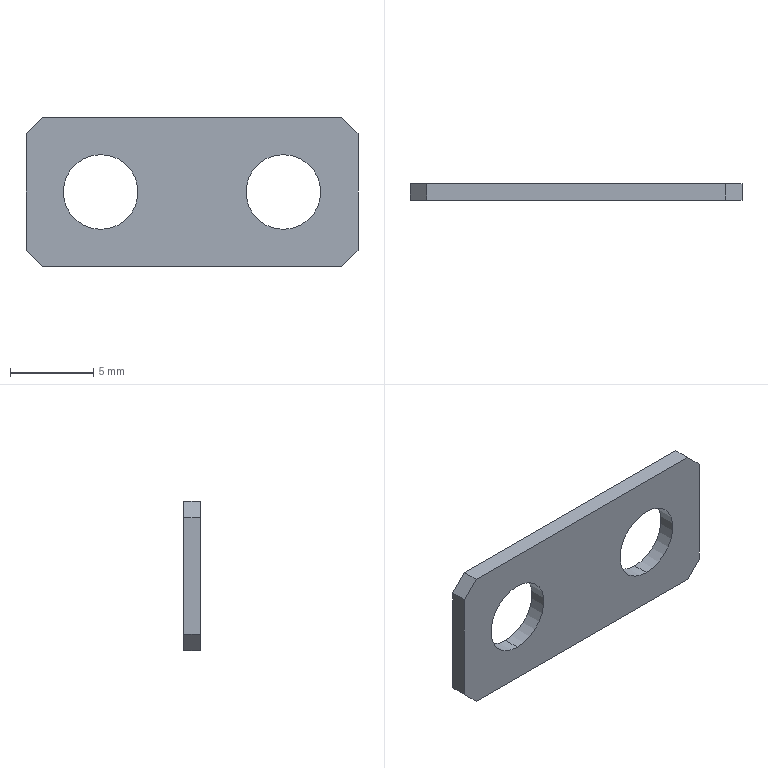Part | STEP file | 10000054028swp000-1 | 1 solid | 14 faces | box 20 x 1 x 9 mm | volume 146.191 mm3 | plane 10 | cylinder 4 | commonest cylinder face diameters 4.5 x4
STEP:
#1=CARTESIAN_POINT('',(-5.5,-0.5,-2.25));
#2=VERTEX_POINT('',#1);
#3=CARTESIAN_POINT('',(-5.5,-0.5,2.25));
#4=VERTEX_POINT('',#3);
#5=CARTESIAN_POINT('',(-5.5,-0.5,0.));
#6=DIRECTION('',(0.,1.,0.));
#7=DIRECTION('',(0.,0.,1.));
#8=AXIS2_PLACEMENT_3D('',#5,#6,#7);
#9=CIRCLE('',#8,2.25);
#10=EDGE_CURVE('',#2,#4,#9,.T.);
#11=ORIENTED_EDGE('',*,*,#10,.F.);
#12=CARTESIAN_POINT('',(-5.5,0.5,-2.25));
#13=VERTEX_POINT('',#12);
#14=CARTESIAN_POINT('',(-5.5,0.5,-2.25));
#15=DIRECTION('',(0.,1.,0.));
#16=VECTOR('',#15,1000.);
#17=LINE('',#14,#16);
#18=EDGE_CURVE('',#2,#13,#17,.T.);
#19=ORIENTED_EDGE('',*,*,#18,.T.);
#20=CARTESIAN_POINT('',(-5.5,0.5,2.25));
#21=VERTEX_POINT('',#20);
#22=CARTESIAN_POINT('',(-5.5,0.5,0.));
#23=DIRECTION('',(0.,1.,0.));
#24=DIRECTION('',(0.,0.,1.));
#25=AXIS2_PLACEMENT_3D('',#22,#23,#24);
#26=CIRCLE('',#25,2.25);
#27=EDGE_CURVE('',#13,#21,#26,.T.);
#28=ORIENTED_EDGE('',*,*,#27,.T.);
#29=CARTESIAN_POINT('',(-5.5,0.5,2.25));
#30=DIRECTION('',(0.,1.,0.));
#31=VECTOR('',#30,1000.);
#32=LINE('',#29,#31);
#33=EDGE_CURVE('',#4,#21,#32,.T.);
#34=ORIENTED_EDGE('',*,*,#33,.F.);
#35=EDGE_LOOP('',(#11,#19,#28,#34));
#36=FACE_OUTER_BOUND('',#35,.T.);
#37=CARTESIAN_POINT('',(-5.5,0.5,0.));
#38=DIRECTION('',(0.,1.,0.));
#39=DIRECTION('',(0.,0.,1.));
#40=AXIS2_PLACEMENT_3D('',#37,#38,#39);
#41=CYLINDRICAL_SURFACE('',#40,2.25);
#42=ADVANCED_FACE('',(#36),#41,.F.);
#43=CARTESIAN_POINT('',(5.5,-0.5,-2.25));
#44=VERTEX_POINT('',#43);
#45=CARTESIAN_POINT('',(5.5,-0.5,2.25));
#46=VERTEX_POINT('',#45);
#47=CARTESIAN_POINT('',(5.5,-0.5,0.));
#48=DIRECTION('',(0.,1.,0.));
#49=DIRECTION('',(0.,0.,1.));
#50=AXIS2_PLACEMENT_3D('',#47,#48,#49);
#51=CIRCLE('',#50,2.25);
#52=EDGE_CURVE('',#44,#46,#51,.T.);
#53=ORIENTED_EDGE('',*,*,#52,.F.);
#54=CARTESIAN_POINT('',(5.5,0.5,-2.25));
#55=VERTEX_POINT('',#54);
#56=CARTESIAN_POINT('',(5.5,0.5,-2.25));
#57=DIRECTION('',(0.,1.,0.));
#58=VECTOR('',#57,1000.);
#59=LINE('',#56,#58);
#60=EDGE_CURVE('',#44,#55,#59,.T.);
#61=ORIENTED_EDGE('',*,*,#60,.T.);
#62=CARTESIAN_POINT('',(5.5,0.5,2.25));
#63=VERTEX_POINT('',#62);
#64=CARTESIAN_POINT('',(5.5,0.5,0.));
#65=DIRECTION('',(0.,1.,0.));
#66=DIRECTION('',(0.,0.,1.));
#67=AXIS2_PLACEMENT_3D('',#64,#65,#66);
#68=CIRCLE('',#67,2.25);
#69=EDGE_CURVE('',#55,#63,#68,.T.);
#70=ORIENTED_EDGE('',*,*,#69,.T.);
#71=CARTESIAN_POINT('',(5.5,0.5,2.25));
#72=DIRECTION('',(0.,1.,0.));
#73=VECTOR('',#72,1000.);
#74=LINE('',#71,#73);
#75=EDGE_CURVE('',#46,#63,#74,.T.);
#76=ORIENTED_EDGE('',*,*,#75,.F.);
#77=EDGE_LOOP('',(#53,#61,#70,#76));
#78=FACE_OUTER_BOUND('',#77,.T.);
#79=CARTESIAN_POINT('',(5.5,0.5,0.));
#80=DIRECTION('',(0.,1.,0.));
#81=DIRECTION('',(0.,0.,1.));
#82=AXIS2_PLACEMENT_3D('',#79,#80,#81);
#83=CYLINDRICAL_SURFACE('',#82,2.25);
#84=ADVANCED_FACE('',(#78),#83,.F.);
#85=CARTESIAN_POINT('',(10.,-0.5,3.5));
#86=VERTEX_POINT('',#85);
#87=CARTESIAN_POINT('',(10.,-0.5,-3.5));
#88=VERTEX_POINT('',#87);
#89=CARTESIAN_POINT('',(10.,-0.5,-4.5));
#90=DIRECTION('',(0.,0.,-1.));
#91=VECTOR('',#90,1000.);
#92=LINE('',#89,#91);
#93=EDGE_CURVE('',#86,#88,#92,.T.);
#94=ORIENTED_EDGE('',*,*,#93,.T.);
#95=CARTESIAN_POINT('',(10.,0.5,-3.5));
#96=VERTEX_POINT('',#95);
#97=CARTESIAN_POINT('',(10.,0.5,-3.5));
#98=DIRECTION('',(0.,1.,0.));
#99=VECTOR('',#98,1000.);
#100=LINE('',#97,#99);
#101=EDGE_CURVE('',#88,#96,#100,.T.);
#102=ORIENTED_EDGE('',*,*,#101,.T.);
#103=CARTESIAN_POINT('',(10.,0.5,3.5));
#104=VERTEX_POINT('',#103);
#105=CARTESIAN_POINT('',(10.,0.5,-4.5));
#106=DIRECTION('',(0.,0.,-1.));
#107=VECTOR('',#106,1000.);
#108=LINE('',#105,#107);
#109=EDGE_CURVE('',#104,#96,#108,.T.);
#110=ORIENTED_EDGE('',*,*,#109,.F.);
#111=CARTESIAN_POINT('',(10.,0.5,3.5));
#112=DIRECTION('',(0.,-1.,0.));
#113=VECTOR('',#112,1000.);
#114=LINE('',#111,#113);
#115=EDGE_CURVE('',#104,#86,#114,.T.);
#116=ORIENTED_EDGE('',*,*,#115,.T.);
#117=EDGE_LOOP('',(#94,#102,#110,#116));
#118=FACE_OUTER_BOUND('',#117,.T.);
#119=CARTESIAN_POINT('',(10.,0.5,-4.5));
#120=DIRECTION('',(-1.,0.,0.));
#121=DIRECTION('',(0.,0.,1.));
#122=AXIS2_PLACEMENT_3D('',#119,#120,#121);
#123=PLANE('',#122);
#124=ADVANCED_FACE('',(#118),#123,.F.);
#125=CARTESIAN_POINT('',(9.,-0.5,-4.5));
#126=VERTEX_POINT('',#125);
#127=CARTESIAN_POINT('',(-9.,-0.5,-4.5));
#128=VERTEX_POINT('',#127);
#129=CARTESIAN_POINT('',(-10.,-0.5,-4.5));
#130=DIRECTION('',(-1.,0.,0.));
#131=VECTOR('',#130,1000.);
#132=LINE('',#129,#131);
#133=EDGE_CURVE('',#126,#128,#132,.T.);
#134=ORIENTED_EDGE('',*,*,#133,.T.);
#135=CARTESIAN_POINT('',(-9.,0.5,-4.5));
#136=VERTEX_POINT('',#135);
#137=CARTESIAN_POINT('',(-9.,0.5,-4.5));
#138=DIRECTION('',(0.,1.,0.));
#139=VECTOR('',#138,1000.);
#140=LINE('',#137,#139);
#141=EDGE_CURVE('',#128,#136,#140,.T.);
#142=ORIENTED_EDGE('',*,*,#141,.T.);
#143=CARTESIAN_POINT('',(9.,0.5,-4.5));
#144=VERTEX_POINT('',#143);
#145=CARTESIAN_POINT('',(-10.,0.5,-4.5));
#146=DIRECTION('',(-1.,0.,0.));
#147=VECTOR('',#146,1000.);
#148=LINE('',#145,#147);
#149=EDGE_CURVE('',#144,#136,#148,.T.);
#150=ORIENTED_EDGE('',*,*,#149,.F.);
#151=CARTESIAN_POINT('',(9.,0.5,-4.5));
#152=DIRECTION('',(0.,-1.,0.));
#153=VECTOR('',#152,1000.);
#154=LINE('',#151,#153);
#155=EDGE_CURVE('',#144,#126,#154,.T.);
#156=ORIENTED_EDGE('',*,*,#155,.T.);
#157=EDGE_LOOP('',(#134,#142,#150,#156));
#158=FACE_OUTER_BOUND('',#157,.T.);
#159=CARTESIAN_POINT('',(-10.,0.5,-4.5));
#160=DIRECTION('',(0.,0.,1.));
#161=DIRECTION('',(1.,0.,0.));
#162=AXIS2_PLACEMENT_3D('',#159,#160,#161);
#163=PLANE('',#162);
#164=ADVANCED_FACE('',(#158),#163,.F.);
#165=CARTESIAN_POINT('',(-10.,0.5,-3.5));
#166=VERTEX_POINT('',#165);
#167=CARTESIAN_POINT('',(-10.,0.5,3.5));
#168=VERTEX_POINT('',#167);
#169=CARTESIAN_POINT('',(-10.,0.5,-4.5));
#170=DIRECTION('',(0.,0.,1.));
#171=VECTOR('',#170,1000.);
#172=LINE('',#169,#171);
#173=EDGE_CURVE('',#166,#168,#172,.T.);
#174=ORIENTED_EDGE('',*,*,#173,.F.);
#175=CARTESIAN_POINT('',(-10.,-0.5,-3.5));
#176=VERTEX_POINT('',#175);
#177=CARTESIAN_POINT('',(-10.,0.5,-3.5));
#178=DIRECTION('',(0.,-1.,0.));
#179=VECTOR('',#178,1000.);
#180=LINE('',#177,#179);
#181=EDGE_CURVE('',#166,#176,#180,.T.);
#182=ORIENTED_EDGE('',*,*,#181,.T.);
#183=CARTESIAN_POINT('',(-10.,-0.5,3.5));
#184=VERTEX_POINT('',#183);
#185=CARTESIAN_POINT('',(-10.,-0.5,-4.5));
#186=DIRECTION('',(0.,0.,1.));
#187=VECTOR('',#186,1000.);
#188=LINE('',#185,#187);
#189=EDGE_CURVE('',#176,#184,#188,.T.);
#190=ORIENTED_EDGE('',*,*,#189,.T.);
#191=CARTESIAN_POINT('',(-10.,0.5,3.5));
#192=DIRECTION('',(0.,1.,0.));
#193=VECTOR('',#192,1000.);
#194=LINE('',#191,#193);
#195=EDGE_CURVE('',#184,#168,#194,.T.);
#196=ORIENTED_EDGE('',*,*,#195,.T.);
#197=EDGE_LOOP('',(#174,#182,#190,#196));
#198=FACE_OUTER_BOUND('',#197,.T.);
#199=CARTESIAN_POINT('',(-10.,0.5,-4.5));
#200=DIRECTION('',(1.,0.,0.));
#201=DIRECTION('',(0.,0.,-1.));
#202=AXIS2_PLACEMENT_3D('',#199,#200,#201);
#203=PLANE('',#202);
#204=ADVANCED_FACE('',(#198),#203,.F.);
#205=CARTESIAN_POINT('',(-9.,0.5,4.5));
#206=VERTEX_POINT('',#205);
#207=CARTESIAN_POINT('',(9.,0.5,4.5));
#208=VERTEX_POINT('',#207);
#209=CARTESIAN_POINT('',(-10.,0.5,4.5));
#210=DIRECTION('',(1.,0.,0.));
#211=VECTOR('',#210,1000.);
#212=LINE('',#209,#211);
#213=EDGE_CURVE('',#206,#208,#212,.T.);
#214=ORIENTED_EDGE('',*,*,#213,.F.);
#215=CARTESIAN_POINT('',(-9.,-0.5,4.5));
#216=VERTEX_POINT('',#215);
#217=CARTESIAN_POINT('',(-9.,0.5,4.5));
#218=DIRECTION('',(0.,-1.,0.));
#219=VECTOR('',#218,1000.);
#220=LINE('',#217,#219);
#221=EDGE_CURVE('',#206,#216,#220,.T.);
#222=ORIENTED_EDGE('',*,*,#221,.T.);
#223=CARTESIAN_POINT('',(9.,-0.5,4.5));
#224=VERTEX_POINT('',#223);
#225=CARTESIAN_POINT('',(-10.,-0.5,4.5));
#226=DIRECTION('',(1.,0.,0.));
#227=VECTOR('',#226,1000.);
#228=LINE('',#225,#227);
#229=EDGE_CURVE('',#216,#224,#228,.T.);
#230=ORIENTED_EDGE('',*,*,#229,.T.);
#231=CARTESIAN_POINT('',(9.,0.5,4.5));
#232=DIRECTION('',(0.,1.,0.));
#233=VECTOR('',#232,1000.);
#234=LINE('',#231,#233);
#235=EDGE_CURVE('',#224,#208,#234,.T.);
#236=ORIENTED_EDGE('',*,*,#235,.T.);
#237=EDGE_LOOP('',(#214,#222,#230,#236));
#238=FACE_OUTER_BOUND('',#237,.T.);
#239=CARTESIAN_POINT('',(-10.,0.5,4.5));
#240=DIRECTION('',(0.,0.,-1.));
#241=DIRECTION('',(-1.,0.,0.));
#242=AXIS2_PLACEMENT_3D('',#239,#240,#241);
#243=PLANE('',#242);
#244=ADVANCED_FACE('',(#238),#243,.F.);
#245=CARTESIAN_POINT('',(-5.5,0.5,0.));
#246=DIRECTION('',(0.,1.,0.));
#247=DIRECTION('',(0.,0.,1.));
#248=AXIS2_PLACEMENT_3D('',#245,#246,#247);
#249=CIRCLE('',#248,2.25);
#250=EDGE_CURVE('',#21,#13,#249,.T.);
#251=ORIENTED_EDGE('',*,*,#250,.F.);
#252=ORIENTED_EDGE('',*,*,#27,.F.);
#253=EDGE_LOOP('',(#251,#252));
#254=FACE_BOUND('',#253,.T.);
#255=CARTESIAN_POINT('',(5.5,0.5,0.));
#256=DIRECTION('',(0.,1.,0.));
#257=DIRECTION('',(0.,0.,1.));
#258=AXIS2_PLACEMENT_3D('',#255,#256,#257);
#259=CIRCLE('',#258,2.25);
#260=EDGE_CURVE('',#63,#55,#259,.T.);
#261=ORIENTED_EDGE('',*,*,#260,.F.);
#262=ORIENTED_EDGE('',*,*,#69,.F.);
#263=EDGE_LOOP('',(#261,#262));
#264=FACE_BOUND('',#263,.T.);
#265=ORIENTED_EDGE('',*,*,#149,.T.);
#266=CARTESIAN_POINT('',(-6.75,0.5,-6.75));
#267=DIRECTION('',(-0.7071,0.,0.7071));
#268=VECTOR('',#267,1000.);
#269=LINE('',#266,#268);
#270=EDGE_CURVE('',#136,#166,#269,.T.);
#271=ORIENTED_EDGE('',*,*,#270,.T.);
#272=ORIENTED_EDGE('',*,*,#173,.T.);
#273=CARTESIAN_POINT('',(-6.75,0.5,6.75));
#274=DIRECTION('',(0.7071,0.,0.7071));
#275=VECTOR('',#274,1000.);
#276=LINE('',#273,#275);
#277=EDGE_CURVE('',#168,#206,#276,.T.);
#278=ORIENTED_EDGE('',*,*,#277,.T.);
#279=ORIENTED_EDGE('',*,*,#213,.T.);
#280=CARTESIAN_POINT('',(6.75,0.5,6.75));
#281=DIRECTION('',(0.7071,0.,-0.7071));
#282=VECTOR('',#281,1000.);
#283=LINE('',#280,#282);
#284=EDGE_CURVE('',#208,#104,#283,.T.);
#285=ORIENTED_EDGE('',*,*,#284,.T.);
#286=ORIENTED_EDGE('',*,*,#109,.T.);
#287=CARTESIAN_POINT('',(6.75,0.5,-6.75));
#288=DIRECTION('',(-0.7071,0.,-0.7071));
#289=VECTOR('',#288,1000.);
#290=LINE('',#287,#289);
#291=EDGE_CURVE('',#96,#144,#290,.T.);
#292=ORIENTED_EDGE('',*,*,#291,.T.);
#293=EDGE_LOOP('',(#265,#271,#272,#278,#279,#285,#286,#292));
#294=FACE_OUTER_BOUND('',#293,.T.);
#295=CARTESIAN_POINT('',(0.,0.5,0.));
#296=DIRECTION('',(0.,1.,0.));
#297=DIRECTION('',(0.,0.,1.));
#298=AXIS2_PLACEMENT_3D('',#295,#296,#297);
#299=PLANE('',#298);
#300=ADVANCED_FACE('',(#254,#264,#294),#299,.T.);
#301=CARTESIAN_POINT('',(-5.5,-0.5,0.));
#302=DIRECTION('',(0.,1.,0.));
#303=DIRECTION('',(0.,0.,1.));
#304=AXIS2_PLACEMENT_3D('',#301,#302,#303);
#305=CIRCLE('',#304,2.25);
#306=EDGE_CURVE('',#4,#2,#305,.T.);
#307=ORIENTED_EDGE('',*,*,#306,.T.);
#308=ORIENTED_EDGE('',*,*,#10,.T.);
#309=EDGE_LOOP('',(#307,#308));
#310=FACE_BOUND('',#309,.T.);
#311=CARTESIAN_POINT('',(5.5,-0.5,0.));
#312=DIRECTION('',(0.,1.,0.));
#313=DIRECTION('',(0.,0.,1.));
#314=AXIS2_PLACEMENT_3D('',#311,#312,#313);
#315=CIRCLE('',#314,2.25);
#316=EDGE_CURVE('',#46,#44,#315,.T.);
#317=ORIENTED_EDGE('',*,*,#316,.T.);
#318=ORIENTED_EDGE('',*,*,#52,.T.);
#319=EDGE_LOOP('',(#317,#318));
#320=FACE_BOUND('',#319,.T.);
#321=ORIENTED_EDGE('',*,*,#189,.F.);
#322=CARTESIAN_POINT('',(-10.,-0.5,-3.5));
#323=DIRECTION('',(0.7071,0.,-0.7071));
#324=VECTOR('',#323,1000.);
#325=LINE('',#322,#324);
#326=EDGE_CURVE('',#176,#128,#325,.T.);
#327=ORIENTED_EDGE('',*,*,#326,.T.);
#328=ORIENTED_EDGE('',*,*,#133,.F.);
#329=CARTESIAN_POINT('',(9.,-0.5,-4.5));
#330=DIRECTION('',(0.7071,0.,0.7071));
#331=VECTOR('',#330,1000.);
#332=LINE('',#329,#331);
#333=EDGE_CURVE('',#126,#88,#332,.T.);
#334=ORIENTED_EDGE('',*,*,#333,.T.);
#335=ORIENTED_EDGE('',*,*,#93,.F.);
#336=CARTESIAN_POINT('',(10.,-0.5,3.5));
#337=DIRECTION('',(-0.7071,0.,0.7071));
#338=VECTOR('',#337,1000.);
#339=LINE('',#336,#338);
#340=EDGE_CURVE('',#86,#224,#339,.T.);
#341=ORIENTED_EDGE('',*,*,#340,.T.);
#342=ORIENTED_EDGE('',*,*,#229,.F.);
#343=CARTESIAN_POINT('',(-9.,-0.5,4.5));
#344=DIRECTION('',(-0.7071,0.,-0.7071));
#345=VECTOR('',#344,1000.);
#346=LINE('',#343,#345);
#347=EDGE_CURVE('',#216,#184,#346,.T.);
#348=ORIENTED_EDGE('',*,*,#347,.T.);
#349=EDGE_LOOP('',(#321,#327,#328,#334,#335,#341,#342,#348));
#350=FACE_OUTER_BOUND('',#349,.T.);
#351=CARTESIAN_POINT('',(0.,-0.5,0.));
#352=DIRECTION('',(0.,1.,0.));
#353=DIRECTION('',(0.,0.,1.));
#354=AXIS2_PLACEMENT_3D('',#351,#352,#353);
#355=PLANE('',#354);
#356=ADVANCED_FACE('',(#310,#320,#350),#355,.F.);
#357=ORIENTED_EDGE('',*,*,#60,.F.);
#358=ORIENTED_EDGE('',*,*,#316,.F.);
#359=ORIENTED_EDGE('',*,*,#75,.T.);
#360=ORIENTED_EDGE('',*,*,#260,.T.);
#361=EDGE_LOOP('',(#357,#358,#359,#360));
#362=FACE_OUTER_BOUND('',#361,.T.);
#363=CARTESIAN_POINT('',(5.5,0.5,0.));
#364=DIRECTION('',(0.,1.,0.));
#365=DIRECTION('',(0.,0.,1.));
#366=AXIS2_PLACEMENT_3D('',#363,#364,#365);
#367=CYLINDRICAL_SURFACE('',#366,2.25);
#368=ADVANCED_FACE('',(#362),#367,.F.);
#369=ORIENTED_EDGE('',*,*,#18,.F.);
#370=ORIENTED_EDGE('',*,*,#306,.F.);
#371=ORIENTED_EDGE('',*,*,#33,.T.);
#372=ORIENTED_EDGE('',*,*,#250,.T.);
#373=EDGE_LOOP('',(#369,#370,#371,#372));
#374=FACE_OUTER_BOUND('',#373,.T.);
#375=CARTESIAN_POINT('',(-5.5,0.5,0.));
#376=DIRECTION('',(0.,1.,0.));
#377=DIRECTION('',(0.,0.,1.));
#378=AXIS2_PLACEMENT_3D('',#375,#376,#377);
#379=CYLINDRICAL_SURFACE('',#378,2.25);
#380=ADVANCED_FACE('',(#374),#379,.F.);
#381=ORIENTED_EDGE('',*,*,#270,.F.);
#382=ORIENTED_EDGE('',*,*,#141,.F.);
#383=ORIENTED_EDGE('',*,*,#326,.F.);
#384=ORIENTED_EDGE('',*,*,#181,.F.);
#385=EDGE_LOOP('',(#381,#382,#383,#384));
#386=FACE_OUTER_BOUND('',#385,.T.);
#387=CARTESIAN_POINT('',(-10.,0.5,-3.5));
#388=DIRECTION('',(0.7071,0.,0.7071));
#389=DIRECTION('',(0.,-1.,0.));
#390=AXIS2_PLACEMENT_3D('',#387,#388,#389);
#391=PLANE('',#390);
#392=ADVANCED_FACE('',(#386),#391,.F.);
#393=ORIENTED_EDGE('',*,*,#277,.F.);
#394=ORIENTED_EDGE('',*,*,#195,.F.);
#395=ORIENTED_EDGE('',*,*,#347,.F.);
#396=ORIENTED_EDGE('',*,*,#221,.F.);
#397=EDGE_LOOP('',(#393,#394,#395,#396));
#398=FACE_OUTER_BOUND('',#397,.T.);
#399=CARTESIAN_POINT('',(-9.,0.5,4.5));
#400=DIRECTION('',(0.7071,0.,-0.7071));
#401=DIRECTION('',(0.,-1.,0.));
#402=AXIS2_PLACEMENT_3D('',#399,#400,#401);
#403=PLANE('',#402);
#404=ADVANCED_FACE('',(#398),#403,.F.);
#405=ORIENTED_EDGE('',*,*,#291,.F.);
#406=ORIENTED_EDGE('',*,*,#101,.F.);
#407=ORIENTED_EDGE('',*,*,#333,.F.);
#408=ORIENTED_EDGE('',*,*,#155,.F.);
#409=EDGE_LOOP('',(#405,#406,#407,#408));
#410=FACE_OUTER_BOUND('',#409,.T.);
#411=CARTESIAN_POINT('',(9.,0.5,-4.5));
#412=DIRECTION('',(-0.7071,0.,0.7071));
#413=DIRECTION('',(0.,-1.,0.));
#414=AXIS2_PLACEMENT_3D('',#411,#412,#413);
#415=PLANE('',#414);
#416=ADVANCED_FACE('',(#410),#415,.F.);
#417=ORIENTED_EDGE('',*,*,#284,.F.);
#418=ORIENTED_EDGE('',*,*,#235,.F.);
#419=ORIENTED_EDGE('',*,*,#340,.F.);
#420=ORIENTED_EDGE('',*,*,#115,.F.);
#421=EDGE_LOOP('',(#417,#418,#419,#420));
#422=FACE_OUTER_BOUND('',#421,.T.);
#423=CARTESIAN_POINT('',(10.,0.5,3.5));
#424=DIRECTION('',(-0.7071,0.,-0.7071));
#425=DIRECTION('',(0.,-1.,0.));
#426=AXIS2_PLACEMENT_3D('',#423,#424,#425);
#427=PLANE('',#426);
#428=ADVANCED_FACE('',(#422),#427,.F.);
#429=CLOSED_SHELL('',(#42,#84,#124,#164,#204,#244,#300,#356,#368,#380,#392,#404,#416,#428));
#430=MANIFOLD_SOLID_BREP('',#429);
#431=CARTESIAN_POINT('',(0.,0.,0.));
#432=DIRECTION('',(0.,0.,1.));
#433=DIRECTION('',(1.,0.,0.));
#434=AXIS2_PLACEMENT_3D('',#431,#432,#433);
#435=(LENGTH_UNIT()NAMED_UNIT(*)SI_UNIT(.MILLI.,.METRE.));
#436=UNCERTAINTY_MEASURE_WITH_UNIT(LENGTH_MEASURE(0.00001),#435,'','');
#437=(NAMED_UNIT(*)PLANE_ANGLE_UNIT()SI_UNIT($,.RADIAN.));
#438=(NAMED_UNIT(*)SI_UNIT($,.STERADIAN.)SOLID_ANGLE_UNIT());
#439=(GEOMETRIC_REPRESENTATION_CONTEXT(3)GLOBAL_UNCERTAINTY_ASSIGNED_CONTEXT((#436))GLOBAL_UNIT_ASSIGNED_CONTEXT((#435,#437,#438))REPRESENTATION_CONTEXT('',''));
#440=ADVANCED_BREP_SHAPE_REPRESENTATION('',(#430,#434),#439);